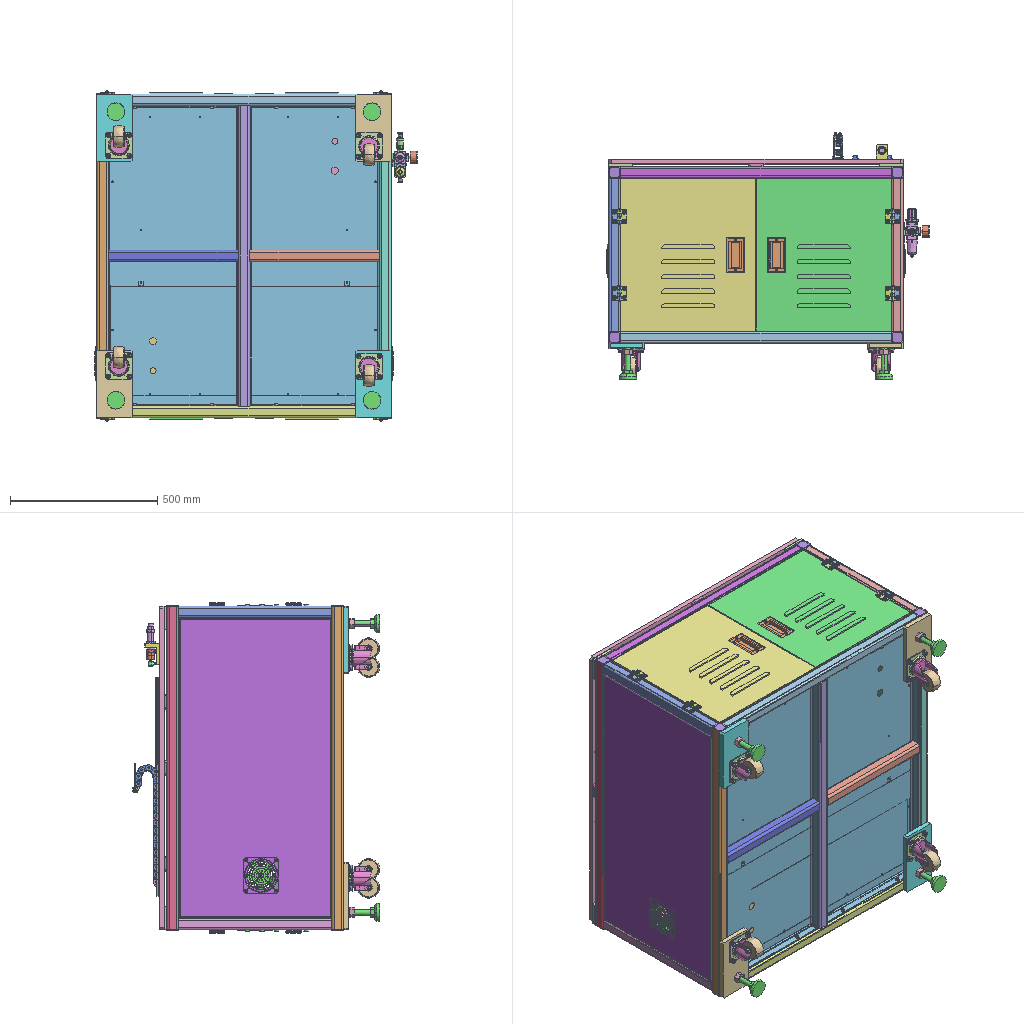Assembly | STEP file | 71 different items | 334 placed | box 1094 x 839 x 1122 mm
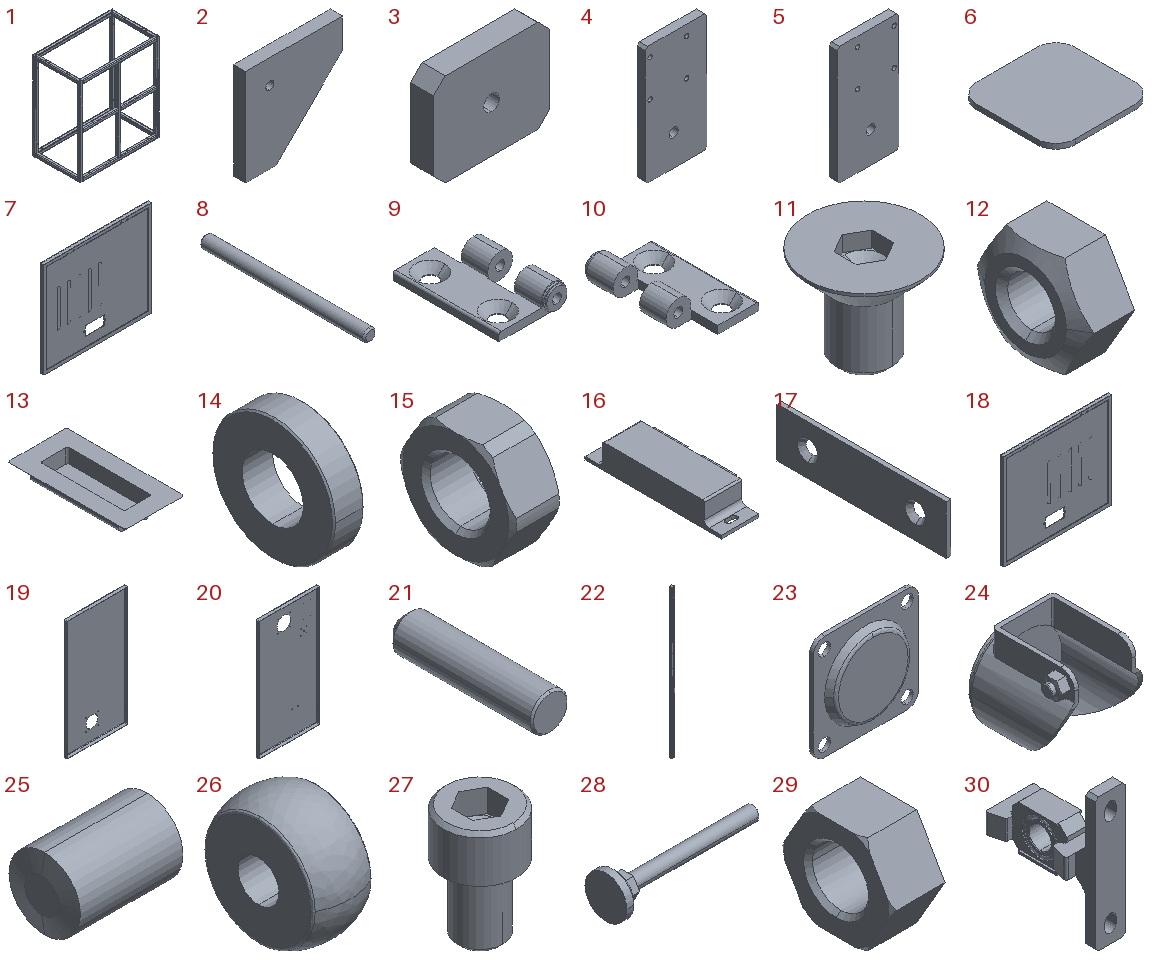Parts list (item | quantity | size | volume):
1 | x1 | 1000 x 600 x 1100 mm | 7334551 mm3
2 | x4 | 80 x 10 x 80 mm | 48512 mm3
3 | x5 | 50 x 10 x 40 mm | 19137 mm3
4 | x4 | 120 x 16 x 230 mm | 433239 mm3
5 | x4 | 120 x 16 x 230 mm | 433239 mm3
6 | x8 | 40 x 40 x 2 mm | 3090 mm3
7 | x2 | 520 x 20 x 460 mm | 497373 mm3
8 | x8 | 4 x 53.4 x 4 mm | 668.164 mm3
9 | x8 | 29.5 x 48.7 x 11 mm | 4677 mm3
10 | x8 | 29.5 x 48.7 x 11 mm | 4677 mm3
11 | x32 | 12 x 12 x 10 mm | 390.282 mm3
12 | x16 | 5 x 11.547 x 10 mm | 323.771 mm3
13 | x4 | 60 x 120 x 15 mm | 28231 mm3
14 | x8 | 2 x 8 x 8 mm | 75.149 mm3
15 | x8 | 3.2 x 7.66 x 7 mm | 92.29 mm3
16 | x8 | 26.5 x 86.5 x 15.5 mm | 25030 mm3
17 | x8 | 1.6 x 55 x 16 mm | 1334 mm3
18 | x2 | 520 x 20 x 460 mm | 497373 mm3
19 | x1 | 520 x 30 x 1020 mm | 905709 mm3
20 | x1 | 520 x 30 x 1020 mm | 901440 mm3
21 | x6 | 4 x 16 x 4 mm | 195.583 mm3
22 | x2 | 15 x 12.5 x 710 mm | 113515 mm3
23 | x4 | 90 x 9.6 x 90 mm | 43068 mm3
24 | x4 | 63.667 x 68.9 x 71.667 mm | 52181 mm3
25 | x4 | 38 x 25 x 25 mm | 18231 mm3
26 | x4 | 36 x 75 x 74.827 mm | 129062 mm3
27 | x16 | 16 x 16 x 25 mm | 2845 mm3
28 | x4 | 211 x 60 x 60 mm | 110948 mm3
29 | x4 | 16 x 34.641 x 30 mm | 8601 mm3
30 | x1 | 23.994 x 51.149 x 66 mm | 13543 mm3
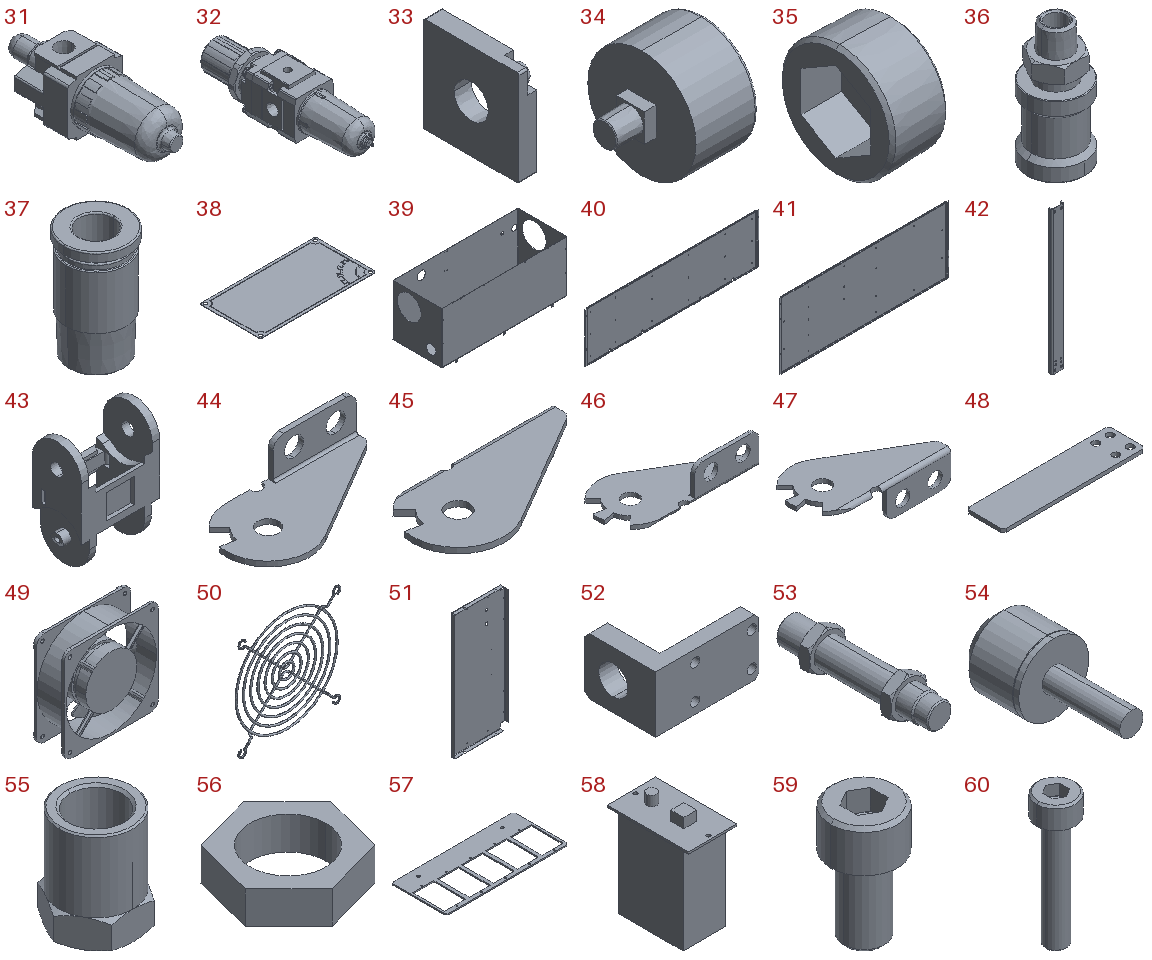31 | x1 | 40 x 119 x 40 mm | 93159 mm3
32 | x1 | 42.5 x 165.1 x 47 mm | 170625 mm3
33 | x2 | 5 x 27.1 x 27.1 mm | 3152 mm3
34 | x1 | 38.5 x 42 x 42 mm | 33324 mm3
35 | x1 | 5 x 9.772 x 9.772 mm | 252.752 mm3
36 | x1 | 26 x 26 x 58 mm | 16455 mm3
37 | x2 | 15 x 15 x 25.7 mm | 2155 mm3
38 | x1 | 126.7 x 66.1 x 0.4 mm | 3280 mm3
39 | x1 | 915 x 360 x 390 mm | 2426206 mm3
40 | x1 | 904 x 7 x 258 mm | 482267 mm3
41 | x1 | 900 x 8 x 353 mm | 657092 mm3
42 | x1 | 38 x 11.5 x 445 mm | 36734 mm3
43 | x19 | 32 x 20 x 45 mm | 6516 mm3
44 | x1 | 40 x 20 x 10 mm | 758.925 mm3
45 | x1 | 40 x 20 x 10 mm | 758.925 mm3
46 | x1 | 40 x 20 x 10 mm | 737.758 mm3
47 | x1 | 40 x 20 x 10 mm | 737.759 mm3
48 | x1 | 100 x 26 x 2.5 mm | 6284 mm3
49 | x2 | 120 x 38.9 x 120 mm | 179083 mm3
50 | x2 | 113.8 x 6.3 x 113.8 mm | 4425 mm3
51 | x2 | 440 x 30 x 1018 mm | 774968 mm3
52 | x1 | 73 x 50 x 40 mm | 44175 mm3
53 | x1 | 26 x 110 x 30.022 mm | 37581 mm3
54 | x1 | 18 x 35.8 x 18 mm | 4359 mm3
55 | x1 | 30.022 x 26 x 35 mm | 9758 mm3
56 | x2 | 28.896 x 29.097 x 8 mm | 2533 mm3
57 | x1 | 315 x 141 x 3 mm | 66219 mm3
58 | x5 | 60 x 100 x 124.5 mm | 482230 mm3
59 | x9 | 13 x 13 x 23 mm | 1660 mm3
60 | x24 | 5.5 x 5.5 x 19 mm | 174.028 mm3
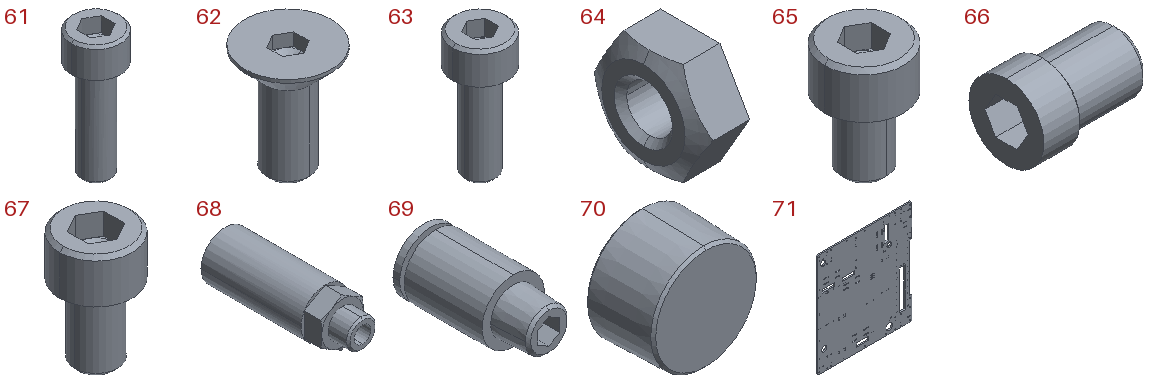61 | x4 | 10 x 10 x 26 mm | 955.225 mm3
62 | x4 | 8 x 8 x 10 mm | 162.002 mm3
63 | x4 | 7 x 7 x 16 mm | 284.727 mm3
64 | x4 | 3.2 x 8.083 x 7 mm | 104.501 mm3
65 | x19 | 7 x 7 x 10 mm | 209.329 mm3
66 | x12 | 15 x 10 x 10 mm | 791.764 mm3
67 | x2 | 10 x 10 x 16 mm | 672.482 mm3
68 | x2 | 22 x 63 x 22 mm | 20442 mm3
69 | x1 | 14 x 28 x 14 mm | 2474 mm3
70 | x3 | 13.263 x 8 x 13.263 mm | 903.778 mm3
71 | x1 | 1000 x 15 x 1100 mm | 15184573 mm3
Placements (level | parent | child | x y z in mm | rotation matrix by rows):
1 | subassembly 2 | subassembly 3 | -0.0 -0.0 -0.0 | 1 0 0 0 1 0 0 0 1
1 | subassembly 2 | subassembly 4 | -460.0 30.0 510.0 | 0 0 -1 0 -1 0 -1 0 0
1 | subassembly 2 | subassembly 4 | -460.0 30.0 -510.0 | 1 0 0 0 -1 0 0 0 -1
1 | subassembly 2 | subassembly 4 | 460.0 30.0 510.0 | -1 0 0 0 -1 0 0 0 1
1 | subassembly 2 | subassembly 4 | 460.0 30.0 -510.0 | 0 0 1 0 -1 0 1 0 0
1 | subassembly 2 | subassembly 5 | -0.0 30.0 -530.0 | 1 0 0 0 -1 0 0 0 -1
1 | subassembly 2 | subassembly 5 | -0.0 30.0 530.0 | -1 0 0 0 -1 0 0 0 1
1 | subassembly 2 | subassembly 5 | 480.0 20.0 -325.0 | 0 0 1 0 1 0 -1 0 0
1 | subassembly 2 | subassembly 5 | 480.0 20.0 225.0 | 0 0 -1 0 1 0 1 0 0
1 | subassembly 2 | subassembly 5 | -480.0 30.0 0.0 | 0 0 -1 0 -1 0 -1 0 0
1 | subassembly 2 | subassembly 6 | -440.0 -596.0 435.0 | -1 0 0 0 1 0 0 0 -1
1 | subassembly 2 | subassembly 6 | 440.0 -596.0 -435.0 | 1 0 0 0 1 0 0 0 1
1 | subassembly 2 | subassembly 7 | -440.0 -596.0 -435.0 | 1 0 0 0 1 0 0 0 1
1 | subassembly 2 | subassembly 7 | 440.0 -596.0 435.0 | -1 0 0 0 1 0 0 0 -1
1 | subassembly 2 | subassembly 8 | 480.0 -0.0 550.0 | 1 0 0 0 1 0 0 0 1
1 | subassembly 2 | subassembly 8 | 480.0 -560.0 550.0 | 1 0 0 0 1 0 0 0 1
1 | subassembly 2 | subassembly 8 | -480.0 -560.0 550.0 | 1 0 0 0 1 0 0 0 1
1 | subassembly 2 | subassembly 8 | -480.0 -0.0 550.0 | 1 0 0 0 1 0 0 0 1
1 | subassembly 2 | subassembly 8 | 480.0 -560.0 -552.0 | -1 0 0 0 -1 0 0 0 1
1 | subassembly 2 | subassembly 8 | 480.0 -0.0 -550.0 | -1 0 0 0 1 0 0 0 -1
1 | subassembly 2 | subassembly 8 | -480.0 -0.0 -552.0 | 0 1 0 -1 0 0 0 0 1
1 | subassembly 2 | subassembly 8 | -480.0 -560.0 -550.0 | -1 0 0 0 1 0 0 0 -1
1 | subassembly 2 | subassembly 9 | 230.0 -280.0 535.0 | 0 0 1 1 0 0 0 1 0
1 | subassembly 2 | subassembly 10 | 464.0 -410.0 555.5 | -0.9918 0 0.128 0 -1 0 0.128 0 0.9918
1 | subassembly 2 | subassembly 11 | 464.0 -410.0 555.5 | -1 0 0 0 -1 0 0 0 1
1 | subassembly 2 | subassembly 12 | 464.0 -410.0 555.5 | -1 0 0 0 -1 0 0 0 1
1 | subassembly 2 | subassembly 13 | 480.0 -425.0 550.2 | -1 0 0 0 -1 0 0 0 1
1 | subassembly 2 | subassembly 13 | 480.0 -395.0 550.2 | -1 0 0 0 -1 0 0 0 1
1 | subassembly 2 | subassembly 13 | 448.0 -395.0 550.2 | -1 0 0 0 -1 0 0 0 1
1 | subassembly 2 | subassembly 13 | 448.0 -425.0 550.2 | -1 0 0 0 -1 0 0 0 1
1 | subassembly 2 | subassembly 14 | 448.0 -425.0 548.8 | 0 0.9997 0.02547 0 -0.02547 0.9997 1 0 0
1 | subassembly 2 | subassembly 14 | 448.0 -395.0 548.8 | 0 0 1 0 -1 0 1 0 0
1 | subassembly 2 | subassembly 10 | 464.0 -150.0 555.5 | -0.9918 0 0.128 0 -1 0 0.128 0 0.9918
1 | subassembly 2 | subassembly 11 | 464.0 -150.0 555.5 | -1 0 0 0 -1 0 0 0 1
1 | subassembly 2 | subassembly 12 | 464.0 -150.0 555.5 | -1 0 0 0 -1 0 0 0 1
1 | subassembly 2 | subassembly 13 | 480.0 -165.0 550.2 | -1 0 0 0 -1 0 0 0 1
1 | subassembly 2 | subassembly 13 | 480.0 -135.0 550.2 | -1 0 0 0 -1 0 0 0 1
1 | subassembly 2 | subassembly 13 | 448.0 -135.0 550.2 | -1 0 0 0 -1 0 0 0 1
1 | subassembly 2 | subassembly 13 | 448.0 -165.0 550.2 | -1 0 0 0 -1 0 0 0 1
1 | subassembly 2 | subassembly 14 | 448.0 -165.0 548.8 | 0 0.9997 0.02547 0 -0.02547 0.9997 1 0 0
1 | subassembly 2 | subassembly 14 | 448.0 -135.0 548.8 | 0 0 1 0 -1 0 1 0 0
1 | subassembly 2 | subassembly 15 | 70.0 -280.0 550.0 | -1 0 0 0 -1 0 0 0 1
1 | subassembly 2 | subassembly 16 | 70.0 -330.0 546.8 | 0 0.723 0.6908 0 0.6908 -0.723 -1 0 0
1 | subassembly 2 | subassembly 17 | 70.0 -330.0 550.0 | 0 -0.4018 0.9157 0 0.9157 0.4018 -1 0 0
1 | subassembly 2 | subassembly 16 | 70.0 -230.0 550.0 | 0 0 1 0 1 0 -1 0 0
1 | subassembly 2 | subassembly 17 | 70.0 -230.0 548.0 | 0 0 1 0 1 0 -1 0 0
1 | subassembly 2 | subassembly 18 | 48.25 -19.5 518.65 | 0 -1 0 0 0 -1 1 0 0
1 | subassembly 2 | subassembly 19 | 48.25 -27.5 533.4 | 0 -1 0 0 0 -1 1 0 0
1 | subassembly 2 | subassembly 18 | 48.25 -540.5 518.65 | 0 1 0 0 0 1 1 0 0
1 | subassembly 2 | subassembly 19 | 48.25 -532.5 533.4 | 0 1 0 0 0 1 1 0 0
1 | subassembly 2 | subassembly 20 | -230.0 -280.0 535.0 | 0 0 -1 -1 0 0 0 1 0
1 | subassembly 2 | subassembly 10 | -464.0 -150.0 555.5 | 0.9918 0 -0.128 0 1 0 0.128 0 0.9918
1 | subassembly 2 | subassembly 11 | -464.0 -150.0 555.5 | 1 0 0 0 1 0 0 0 1
1 | subassembly 2 | subassembly 12 | -464.0 -150.0 555.5 | 1 0 0 0 1 0 0 0 1
1 | subassembly 2 | subassembly 13 | -480.0 -135.0 550.2 | 1 0 0 0 1 0 0 0 1
1 | subassembly 2 | subassembly 13 | -480.0 -165.0 550.2 | 1 0 0 0 1 0 0 0 1
1 | subassembly 2 | subassembly 13 | -448.0 -165.0 550.2 | 1 0 0 0 1 0 0 0 1
1 | subassembly 2 | subassembly 13 | -448.0 -135.0 550.2 | 1 0 0 0 1 0 0 0 1
1 | subassembly 2 | subassembly 14 | -448.0 -135.0 548.8 | 0 -0.9997 -0.02547 0 0.02547 -0.9997 1 0 0
1 | subassembly 2 | subassembly 14 | -448.0 -165.0 548.8 | 0 0 -1 0 1 0 1 0 0
1 | subassembly 2 | subassembly 10 | -464.0 -410.0 555.5 | 0.9918 0 -0.128 0 1 0 0.128 0 0.9918
1 | subassembly 2 | subassembly 11 | -464.0 -410.0 555.5 | 1 0 0 0 1 0 0 0 1
1 | subassembly 2 | subassembly 12 | -464.0 -410.0 555.5 | 1 0 0 0 1 0 0 0 1
1 | subassembly 2 | subassembly 13 | -480.0 -395.0 550.2 | 1 0 0 0 1 0 0 0 1
1 | subassembly 2 | subassembly 13 | -480.0 -425.0 550.2 | 1 0 0 0 1 0 0 0 1
1 | subassembly 2 | subassembly 13 | -448.0 -425.0 550.2 | 1 0 0 0 1 0 0 0 1
1 | subassembly 2 | subassembly 13 | -448.0 -395.0 550.2 | 1 0 0 0 1 0 0 0 1
1 | subassembly 2 | subassembly 14 | -448.0 -395.0 548.8 | 0 -0.9997 -0.02547 0 0.02547 -0.9997 1 0 0
1 | subassembly 2 | subassembly 14 | -448.0 -425.0 548.8 | 0 0 -1 0 1 0 1 0 0
1 | subassembly 2 | subassembly 15 | -70.0 -280.0 550.0 | 1 0 0 0 1 0 0 0 1
1 | subassembly 2 | subassembly 16 | -70.0 -230.0 546.8 | 0 -0.723 -0.6908 0 -0.6908 0.723 -1 0 0
1 | subassembly 2 | subassembly 17 | -70.0 -230.0 550.0 | 0 0.4018 -0.9157 0 -0.9157 -0.4018 -1 0 0
1 | subassembly 2 | subassembly 16 | -70.0 -330.0 550.0 | 0 0 -1 0 -1 0 -1 0 0
1 | subassembly 2 | subassembly 17 | -70.0 -330.0 548.0 | 0 0 -1 0 -1 0 -1 0 0
1 | subassembly 2 | subassembly 18 | -48.25 -540.5 518.65 | 0 1 0 0 0 1 1 0 0
1 | subassembly 2 | subassembly 19 | -48.25 -532.5 533.4 | 0 1 0 0 0 1 1 0 0
1 | subassembly 2 | subassembly 18 | -48.25 -19.5 518.65 | 0 -1 0 0 0 -1 1 0 0
1 | subassembly 2 | subassembly 19 | -48.25 -27.5 533.4 | 0 -1 0 0 0 -1 1 0 0
1 | subassembly 2 | subassembly 9 | -230.0 -280.0 -535.0 | 0 0 -1 1 0 0 0 -1 0
1 | subassembly 2 | subassembly 10 | -464.0 -410.0 -555.5 | 0.9918 0 -0.128 0 -1 0 -0.128 0 -0.9918
1 | subassembly 2 | subassembly 11 | -464.0 -410.0 -555.5 | 1 0 0 0 -1 0 0 0 -1
1 | subassembly 2 | subassembly 12 | -464.0 -410.0 -555.5 | 1 0 0 0 -1 0 0 0 -1
1 | subassembly 2 | subassembly 13 | -480.0 -425.0 -550.2 | 1 0 0 0 -1 0 0 0 -1
1 | subassembly 2 | subassembly 13 | -480.0 -395.0 -550.2 | 1 0 0 0 -1 0 0 0 -1
1 | subassembly 2 | subassembly 13 | -448.0 -395.0 -550.2 | 1 0 0 0 -1 0 0 0 -1
1 | subassembly 2 | subassembly 13 | -448.0 -425.0 -550.2 | 1 0 0 0 -1 0 0 0 -1
1 | subassembly 2 | subassembly 14 | -448.0 -425.0 -548.8 | 0 -0.9997 -0.02547 0 -0.02547 0.9997 -1 0 0
1 | subassembly 2 | subassembly 14 | -448.0 -395.0 -548.8 | 0 0 -1 0 -1 0 -1 0 0
1 | subassembly 2 | subassembly 10 | -464.0 -150.0 -555.5 | 0.9918 0 -0.128 0 -1 0 -0.128 0 -0.9918
1 | subassembly 2 | subassembly 11 | -464.0 -150.0 -555.5 | 1 0 0 0 -1 0 0 0 -1
1 | subassembly 2 | subassembly 12 | -464.0 -150.0 -555.5 | 1 0 0 0 -1 0 0 0 -1
1 | subassembly 2 | subassembly 13 | -480.0 -165.0 -550.2 | 1 0 0 0 -1 0 0 0 -1
1 | subassembly 2 | subassembly 13 | -480.0 -135.0 -550.2 | 1 0 0 0 -1 0 0 0 -1
1 | subassembly 2 | subassembly 13 | -448.0 -135.0 -550.2 | 1 0 0 0 -1 0 0 0 -1
1 | subassembly 2 | subassembly 13 | -448.0 -165.0 -550.2 | 1 0 0 0 -1 0 0 0 -1
1 | subassembly 2 | subassembly 14 | -448.0 -165.0 -548.8 | 0 -0.9997 -0.02547 0 -0.02547 0.9997 -1 0 0
1 | subassembly 2 | subassembly 14 | -448.0 -135.0 -548.8 | 0 0 -1 0 -1 0 -1 0 0
1 | subassembly 2 | subassembly 15 | -70.0 -280.0 -550.0 | 1 0 0 0 -1 0 0 0 -1
1 | subassembly 2 | subassembly 16 | -70.0 -330.0 -546.8 | 0 -0.723 -0.6908 0 0.6908 -0.723 1 0 0
1 | subassembly 2 | subassembly 17 | -70.0 -330.0 -550.0 | 0 0.4018 -0.9157 0 0.9157 0.4018 1 0 0
1 | subassembly 2 | subassembly 16 | -70.0 -230.0 -550.0 | 0 0 -1 0 1 0 1 0 0
1 | subassembly 2 | subassembly 17 | -70.0 -230.0 -548.0 | 0 0 -1 0 1 0 1 0 0
1 | subassembly 2 | subassembly 18 | -48.25 -19.5 -518.65 | 0 1 0 0 0 -1 -1 0 0
1 | subassembly 2 | subassembly 19 | -48.25 -27.5 -533.4 | 0 1 0 0 0 -1 -1 0 0
1 | subassembly 2 | subassembly 18 | -48.25 -540.5 -518.65 | 0 -1 0 0 0 1 -1 0 0
1 | subassembly 2 | subassembly 19 | -48.25 -532.5 -533.4 | 0 -1 0 0 0 1 -1 0 0
1 | subassembly 2 | subassembly 20 | 230.0 -280.0 -535.0 | 0 0 1 -1 0 0 0 -1 0
1 | subassembly 2 | subassembly 10 | 464.0 -150.0 -555.5 | -0.9918 0 0.128 0 1 0 -0.128 0 -0.9918
1 | subassembly 2 | subassembly 11 | 464.0 -150.0 -555.5 | -1 0 0 0 1 0 0 0 -1
1 | subassembly 2 | subassembly 12 | 464.0 -150.0 -555.5 | -1 0 0 0 1 0 0 0 -1
1 | subassembly 2 | subassembly 13 | 480.0 -135.0 -550.2 | -1 0 0 0 1 0 0 0 -1
1 | subassembly 2 | subassembly 13 | 480.0 -165.0 -550.2 | -1 0 0 0 1 0 0 0 -1
1 | subassembly 2 | subassembly 13 | 448.0 -165.0 -550.2 | -1 0 0 0 1 0 0 0 -1
1 | subassembly 2 | subassembly 13 | 448.0 -135.0 -550.2 | -1 0 0 0 1 0 0 0 -1
1 | subassembly 2 | subassembly 14 | 448.0 -135.0 -548.8 | 0 0.9997 0.02547 0 0.02547 -0.9997 -1 0 0
1 | subassembly 2 | subassembly 14 | 448.0 -165.0 -548.8 | 0 0 1 0 1 0 -1 0 0
1 | subassembly 2 | subassembly 10 | 464.0 -410.0 -555.5 | -0.9918 0 0.128 0 1 0 -0.128 0 -0.9918
1 | subassembly 2 | subassembly 11 | 464.0 -410.0 -555.5 | -1 0 0 0 1 0 0 0 -1
1 | subassembly 2 | subassembly 12 | 464.0 -410.0 -555.5 | -1 0 0 0 1 0 0 0 -1
1 | subassembly 2 | subassembly 13 | 480.0 -395.0 -550.2 | -1 0 0 0 1 0 0 0 -1
1 | subassembly 2 | subassembly 13 | 480.0 -425.0 -550.2 | -1 0 0 0 1 0 0 0 -1
1 | subassembly 2 | subassembly 13 | 448.0 -425.0 -550.2 | -1 0 0 0 1 0 0 0 -1
1 | subassembly 2 | subassembly 13 | 448.0 -395.0 -550.2 | -1 0 0 0 1 0 0 0 -1
1 | subassembly 2 | subassembly 14 | 448.0 -395.0 -548.8 | 0 0.9997 0.02547 0 0.02547 -0.9997 -1 0 0
1 | subassembly 2 | subassembly 14 | 448.0 -425.0 -548.8 | 0 0 1 0 1 0 -1 0 0
1 | subassembly 2 | subassembly 15 | 70.0 -280.0 -550.0 | -1 0 0 0 1 0 0 0 -1
1 | subassembly 2 | subassembly 16 | 70.0 -230.0 -546.8 | 0 0.723 0.6908 0 -0.6908 0.723 1 0 0
1 | subassembly 2 | subassembly 17 | 70.0 -230.0 -550.0 | 0 -0.4018 0.9157 0 -0.9157 -0.4018 1 0 0
1 | subassembly 2 | subassembly 16 | 70.0 -330.0 -550.0 | 0 0 1 0 -1 0 1 0 0
1 | subassembly 2 | subassembly 17 | 70.0 -330.0 -548.0 | 0 0 1 0 -1 0 1 0 0
1 | subassembly 2 | subassembly 18 | 48.25 -540.5 -518.65 | 0 -1 0 0 0 1 -1 0 0
1 | subassembly 2 | subassembly 19 | 48.25 -532.5 -533.4 | 0 -1 0 0 0 1 -1 0 0
1 | subassembly 2 | subassembly 18 | 48.25 -19.5 -518.65 | 0 1 0 0 0 -1 -1 0 0
1 | subassembly 2 | subassembly 19 | 48.25 -27.5 -533.4 | 0 1 0 0 0 -1 -1 0 0
1 | subassembly 2 | subassembly 21 | -470.0 -280.0 -0.0 | 0 -1 0 1 0 0 0 0 1
1 | subassembly 2 | subassembly 22 | 470.0 -280.0 -0.0 | 0 1 0 1 0 0 0 0 -1
1 | subassembly 2 | subassembly 23 | 462.0 33.0 -385.0 | 0.9252 0 0.3796 0 1 0 -0.3796 0 0.9252
1 | subassembly 2 | subassembly 23 | 346.0 33.0 -385.0 | 0.9252 0 0.3796 0 1 0 -0.3796 0 0.9252
1 | subassembly 2 | subassembly 23 | 346.0 33.0 -75.0 | 1 0 0 0 1 0 0 0 1
1 | subassembly 2 | subassembly 23 | 346.0 33.0 235.0 | 1 0 0 0 1 0 0 0 1
1 | subassembly 2 | subassembly 23 | 462.0 33.0 -75.0 | 1 0 0 0 1 0 0 0 1
1 | subassembly 2 | subassembly 23 | 462.0 33.0 235.0 | 1 0 0 0 1 0 0 0 1
1 | subassembly 2 | subassembly 24 | 452.5 69.0 -363.0 | 1 0 0 0 1 0 0 0 1
1 | subassembly 2 | subassembly 24 | 336.5 69.0 -363.0 | 1 0 0 0 1 0 0 0 1
1 | subassembly 2 | subassembly 6 | 440.0 -596.0 -435.0 | 1 0 0 0 1 0 0 0 1
1 | subassembly 2 | subassembly 25 | 425.0 -596.0 -375.866 | -1 0 0 0 1 0 0 0 -1
1 | subassembly 2 | subassembly 26 | 425.0 -596.0 -375.866 | -1 0 0 0 1 0 0 0 -1
1 | subassembly 2 | subassembly 27 | 425.0 -664.5 -405.866 | 1 0 0 0 -1 0 0 0 -1
1 | subassembly 2 | subassembly 28 | 425.0 -664.5 -405.866 | -1 0 0 0 1 0 0 0 -1
1 | subassembly 2 | subassembly 29 | 389.5 -599.2 -411.366 | -1 0 0 0 0 -1 0 -1 0
1 | subassembly 2 | subassembly 29 | 389.5 -599.2 -340.366 | -1 0 0 0 0 -1 0 -1 0
1 | subassembly 2 | subassembly 29 | 460.5 -599.2 -340.366 | -1 0 0 0 0 -1 0 -1 0
1 | subassembly 2 | subassembly 29 | 460.5 -599.2 -411.366 | -1 0 0 0 0 -1 0 -1 0
1 | subassembly 2 | subassembly 30 | 435.0 -702.0 -490.0 | 0 0.9914 0.1311 1 0 0 0 0.1311 -0.9914
1 | subassembly 2 | subassembly 31 | 435.0 -617.0 -490.0 | 0 0.987 0.1607 1 0 0 0 0.1607 -0.987
1 | subassembly 2 | subassembly 7 | 440.0 -596.0 435.0 | -1 0 0 0 1 0 0 0 -1
1 | subassembly 2 | subassembly 25 | 425.0 -596.0 373.5 | -1 0 0 0 1 0 0 0 -1
1 | subassembly 2 | subassembly 26 | 425.0 -596.0 373.5 | -1 0 0 0 1 0 0 0 -1
1 | subassembly 2 | subassembly 27 | 425.0 -664.5 343.5 | 1 0 0 0 -1 0 0 0 -1
1 | subassembly 2 | subassembly 28 | 425.0 -664.5 343.5 | -1 0 0 0 1 0 0 0 -1
1 | subassembly 2 | subassembly 29 | 389.5 -599.2 338.0 | -1 0 0 0 0 -1 0 -1 0
1 | subassembly 2 | subassembly 29 | 389.5 -599.2 409.0 | -1 0 0 0 0 -1 0 -1 0
1 | subassembly 2 | subassembly 29 | 460.5 -599.2 409.0 | -1 0 0 0 0 -1 0 -1 0
1 | subassembly 2 | subassembly 29 | 460.5 -599.2 338.0 | -1 0 0 0 0 -1 0 -1 0
1 | subassembly 2 | subassembly 30 | 435.0 -702.0 490.0 | 0 0 1 1 0 0 0 1 0
1 | subassembly 2 | subassembly 31 | 435.0 -617.0 490.0 | 0 -0.02991 0.9996 1 0 0 0 0.9996 0.02991
1 | subassembly 2 | subassembly 6 | -440.0 -596.0 435.0 | -1 0 0 0 1 0 0 0 -1
1 | subassembly 2 | subassembly 25 | -425.0 -596.0 375.866 | 1 0 0 0 1 0 0 0 1
1 | subassembly 2 | subassembly 26 | -425.0 -596.0 375.866 | 1 0 0 0 1 0 0 0 1
1 | subassembly 2 | subassembly 27 | -425.0 -664.5 405.866 | -1 0 0 0 -1 0 0 0 1
1 | subassembly 2 | subassembly 28 | -425.0 -664.5 405.866 | 1 0 0 0 1 0 0 0 1
1 | subassembly 2 | subassembly 29 | -389.5 -599.2 411.366 | 1 0 0 0 0 -1 0 1 0
1 | subassembly 2 | subassembly 29 | -389.5 -599.2 340.366 | 1 0 0 0 0 -1 0 1 0
1 | subassembly 2 | subassembly 29 | -460.5 -599.2 340.366 | 1 0 0 0 0 -1 0 1 0
1 | subassembly 2 | subassembly 29 | -460.5 -599.2 411.366 | 1 0 0 0 0 -1 0 1 0
1 | subassembly 2 | subassembly 30 | -435.0 -702.0 490.0 | 0 -0.9914 -0.1311 1 0 0 0 -0.1311 0.9914
1 | subassembly 2 | subassembly 31 | -435.0 -617.0 490.0 | 0 -0.987 -0.1607 1 0 0 0 -0.1607 0.987
1 | subassembly 2 | subassembly 7 | -440.0 -596.0 -435.0 | 1 0 0 0 1 0 0 0 1
1 | subassembly 2 | subassembly 25 | -425.0 -596.0 -373.5 | 1 0 0 0 1 0 0 0 1
1 | subassembly 2 | subassembly 26 | -425.0 -596.0 -373.5 | 1 0 0 0 1 0 0 0 1
1 | subassembly 2 | subassembly 27 | -425.0 -664.5 -343.5 | -1 0 0 0 -1 0 0 0 1
1 | subassembly 2 | subassembly 28 | -425.0 -664.5 -343.5 | 1 0 0 0 1 0 0 0 1
1 | subassembly 2 | subassembly 29 | -389.5 -599.2 -338.0 | 1 0 0 0 0 -1 0 1 0
1 | subassembly 2 | subassembly 29 | -389.5 -599.2 -409.0 | 1 0 0 0 0 -1 0 1 0
1 | subassembly 2 | subassembly 29 | -460.5 -599.2 -409.0 | 1 0 0 0 0 -1 0 1 0
1 | subassembly 2 | subassembly 29 | -460.5 -599.2 -338.0 | 1 0 0 0 0 -1 0 1 0
1 | subassembly 2 | subassembly 30 | -435.0 -702.0 -490.0 | 0 0 -1 1 0 0 0 -1 0
1 | subassembly 2 | subassembly 31 | -435.0 -617.0 -490.0 | 0 0.02991 -0.9996 1 0 0 0 -0.9996 -0.02991
1 | subassembly 2 | subassembly 32 | 500.0 -203.5 310.0 | 0 1 0 0 0 -1 -1 0 0
1 | subassembly 2 | subassembly 33 | 530.0 -226.5 285.0 | 1 0 0 0 1 0 0 0 1
1 | subassembly 2 | subassembly 34 | 530.0 -171.0 335.0 | 0 0 1 0 1 0 -1 0 0
1 | subassembly 2 | subassembly 35 | 558.5 -199.5 335.0 | 1 0 0 0 1 0 0 0 1
1 | subassembly 2 | subassembly 36 | 588.0 -199.5 335.0 | 1 0 0 0 1 0 0 0 1
1 | subassembly 2 | subassembly 35 | 501.5 -199.5 335.0 | -1 0 0 0 -1 0 0 0 1
1 | subassembly 2 | subassembly 37 | 502.0 -199.5 335.0 | 1 0 0 0 1 0 0 0 1
1 | subassembly 2 | subassembly 38 | 530.0 -203.5 343.5 | -0.9347 -0.3555 0 -0.3555 0.9347 0 0 0 -1
1 | subassembly 2 | subassembly 39 | 530.0 -203.5 392.5 | 1 0 0 0 1 0 0 0 1
1 | subassembly 2 | subassembly 39 | 530.0 -203.5 274.0 | -0.9237 -0.383 0 -0.383 0.9237 0 0 0 -1
1 | subassembly 2 | subassembly 40 | 500.4 -103.05 -366.65 | 0 0 1 0 1 0 -1 0 0
1 | subassembly 2 | subassembly 41 | -0.0 -360.0 -100.0 | -1 0 0 0 1 0 0 0 -1
1 | subassembly 2 | subassembly 42 | -0.0 -531.0 -348.0 | 1 0 0 0 1 0 0 0 1
1 | subassembly 2 | subassembly 43 | -0.0 -360.0 -110.0 | 1 0 0 0 0 1 0 -1 0
1 | subassembly 2 | subassembly 44 | 278.0 46.5 -212.5 | 1 0 0 0 1 0 0 0 1
1 | subassembly 2 | subassembly 45 | 278.0 116.5 -63.443 | 1 0 0 0 -1 0 0 0 -1
1 | subassembly 2 | subassembly 45 | 278.0 120.667 -37.533 | 1 0 0 0 -0.9091 0.4167 0 -0.4167 -0.9091
1 | subassembly 2 | subassembly 45 | 278.0 115.69 -8.494 | 1 0 0 0 -0.2778 0.9606 0 -0.9606 -0.2778
1 | subassembly 2 | subassembly 45 | 278.0 90.442 6.692 | 1 0 0 0 0.5464 0.8375 0 -0.8375 0.5464
1 | subassembly 2 | subassembly 45 | 278.0 62.981 -2.605 | 1 0 0 0 0.9827 0.1852 0 -0.1852 0.9827
1 | subassembly 2 | subassembly 45 | 278.0 56.5 -27.0 | 1 0 0 0 1 0 0 0 1
1 | subassembly 2 | subassembly 45 | 278.0 56.5 -52.0 | 1 0 0 0 1 0 0 0 1
1 | subassembly 2 | subassembly 45 | 278.0 56.5 -77.0 | 1 0 0 0 1 0 0 0 1
1 | subassembly 2 | subassembly 45 | 278.0 56.5 -102.0 | 1 0 0 0 1 0 0 0 1
1 | subassembly 2 | subassembly 45 | 278.0 56.5 -127.0 | 1 0 0 0 1 0 0 0 1
1 | subassembly 2 | subassembly 45 | 278.0 56.5 -152.0 | 1 0 0 0 1 0 0 0 1
1 | subassembly 2 | subassembly 45 | 278.0 56.5 -177.0 | 1 0 0 0 1 0 0 0 1
1 | subassembly 2 | subassembly 45 | 278.0 56.5 -202.0 | 1 0 0 0 1 0 0 0 1
1 | subassembly 2 | subassembly 45 | 278.0 56.5 -227.0 | 1 0 0 0 1 0 0 0 1
1 | subassembly 2 | subassembly 45 | 278.0 56.5 -252.0 | 1 0 0 0 1 0 0 0 1
1 | subassembly 2 | subassembly 45 | 278.0 56.5 -277.0 | 1 0 0 0 1 0 0 0 1
1 | subassembly 2 | subassembly 45 | 278.0 56.5 -302.0 | 1 0 0 0 1 0 0 0 1
1 | subassembly 2 | subassembly 45 | 278.0 56.5 -327.0 | 1 0 0 0 1 0 0 0 1
1 | subassembly 2 | subassembly 45 | 278.0 56.5 -352.0 | 1 0 0 0 1 0 0 0 1
1 | subassembly 2 | subassembly 46 | 291.9 66.5 -387.0 | 0 0 -1 0 -1 0 -1 0 0
1 | subassembly 2 | subassembly 47 | 264.1 66.5 -387.0 | 0 0 -1 0 -1 0 -1 0 0
1 | subassembly 2 | subassembly 48 | 291.0 126.5 -53.443 | 0 0 -1 0 -1 0 -1 0 0
1 | subassembly 2 | subassembly 49 | 265.0 126.5 -53.443 | 0 0 -1 0 -1 0 -1 0 0
1 | subassembly 2 | subassembly 50 | 278.0 126.5 -33.443 | 0 -1 0 0 0 1 -1 0 0
1 | subassembly 2 | subassembly 51 | 487.6 -300.0 -365.0 | 0 1 0 0 0 -1 -1 0 0
1 | subassembly 2 | subassembly 52 | 489.6 -300.0 -365.0 | 0 1 0 0 0 -1 -1 0 0
1 | subassembly 2 | subassembly 51 | -487.6 -300.0 -365.0 | 0 -1 0 1 0 0 0 0 1
1 | subassembly 2 | subassembly 52 | -489.6 -300.0 -365.0 | 0 -1 0 1 0 0 0 0 1
1 | subassembly 2 | subassembly 53 | 240.0 -570.0 1.0 | 1 0 0 0 1 0 0 0 1
1 | subassembly 2 | subassembly 53 | -240.0 -570.0 -0.0 | -1 0 0 0 1 0 0 0 -1
1 | subassembly 2 | subassembly 54 | 428.0 55.0 410.0 | 0 0 1 0 1 0 -1 0 0
1 | subassembly 2 | subassembly 55 | 428.0 75.0 492.0 | 0.1382 0 0.9904 -0.9904 0 0.1382 0 -1 0
1 | subassembly 2 | subassembly 56 | 428.0 75.0 492.0 | 0.1382 0 0.9904 -0.9904 0 0.1382 0 -1 0
1 | subassembly 2 | subassembly 57 | 428.0 75.0 384.5 | 0.1382 -0.9904 0 -0.9904 -0.1382 0 0 0 -1
1 | subassembly 2 | subassembly 58 | 428.0 75.0 418.0 | -0.07756 -0.997 0 -0.997 0.07756 0 0 0 -1
1 | subassembly 2 | subassembly 58 | 428.0 75.0 431.0 | -1 0 0 0 1 0 0 0 -1
1 | subassembly 2 | subassembly 59 | -293.5 -40.0 -507.0 | -1 0 0 0 1 0 0 0 -1
1 | subassembly 2 | subassembly 60 | -169.0 -71.0 -510.0 | -1 0 0 0 1 0 0 0 -1
1 | subassembly 2 | subassembly 60 | -231.0 -71.0 -510.0 | -1 0 0 0 1 0 0 0 -1
1 | subassembly 2 | subassembly 60 | -293.0 -71.0 -510.0 | -1 0 0 0 1 0 0 0 -1
1 | subassembly 2 | subassembly 60 | -355.0 -71.0 -510.0 | -1 0 0 0 1 0 0 0 -1
1 | subassembly 2 | subassembly 60 | -417.0 -71.0 -510.0 | -1 0 0 0 1 0 0 0 -1
1 | subassembly 2 | subassembly 61 | 480.0 36.4 530.0 | 1 0 0 0 0 1 0 -1 0
1 | subassembly 2 | subassembly 61 | -480.0 36.4 -530.0 | 1 0 0 0 0 1 0 -1 0
1 | subassembly 2 | subassembly 61 | -0.0 36.4 -530.0 | 1 0 0 0 0 1 0 -1 0
1 | subassembly 2 | subassembly 61 | 480.0 36.4 -325.0 | 1 0 0 0 0 1 0 -1 0
1 | subassembly 2 | subassembly 61 | -0.0 36.4 530.0 | 1 0 0 0 0 1 0 -1 0
1 | subassembly 2 | subassembly 61 | -480.0 36.4 -0.0 | 1 0 0 0 0 1 0 -1 0
1 | subassembly 2 | subassembly 61 | -480.0 36.4 530.0 | 1 0 0 0 0 1 0 -1 0
1 | subassembly 2 | subassembly 61 | 480.0 36.4 225.0 | 1 0 0 0 0 1 0 -1 0
1 | subassembly 2 | subassembly 61 | 480.0 36.4 -530.0 | 1 0 0 0 0 1 0 -1 0
1 | subassembly 2 | subassembly 62 | 336.5 53.0 -388.0 | 0.326 -0.9454 0 0 0 1 -0.9454 -0.326 0
1 | subassembly 2 | subassembly 62 | 452.5 53.0 -388.0 | 0.326 -0.9454 0 0 0 1 -0.9454 -0.326 0
1 | subassembly 2 | subassembly 63 | 416.0 55.0 355.0 | 0.9391 -0.3436 0 0 0 1 -0.3436 -0.9391 0
1 | subassembly 2 | subassembly 63 | 440.0 55.0 355.0 | 0.9391 -0.3436 0 0 0 1 -0.3436 -0.9391 0
1 | subassembly 2 | subassembly 63 | 440.0 55.0 395.0 | 0.9391 -0.3436 0 0 0 1 -0.3436 -0.9391 0
1 | subassembly 2 | subassembly 63 | 416.0 55.0 395.0 | 0.9391 -0.3436 0 0 0 1 -0.3436 -0.9391 0
1 | subassembly 2 | subassembly 64 | 268.0 44.2 -425.0 | 0.7216 0.6923 0 0 0 1 0.6923 -0.7216 0
1 | subassembly 2 | subassembly 64 | 288.0 44.2 -425.0 | 0.7216 0.6923 0 0 0 1 0.6923 -0.7216 0
1 | subassembly 2 | subassembly 64 | 288.0 44.2 -0.0 | 0.7216 0.6923 0 0 0 1 0.6923 -0.7216 0
1 | subassembly 2 | subassembly 64 | 268.0 44.2 0.0 | 0.7216 0.6923 0 0 0 1 0.6923 -0.7216 0
1 | subassembly 2 | subassembly 65 | 285.0 125.3 -78.443 | -0.3569 -0.9341 0 0 0 -1 0.9341 -0.3569 0
1 | subassembly 2 | subassembly 65 | 271.0 125.3 -78.443 | -0.3569 -0.9341 0 0 0 -1 0.9341 -0.3569 0
1 | subassembly 2 | subassembly 65 | 285.0 125.3 -68.443 | -0.3569 -0.9341 0 0 0 -1 0.9341 -0.3569 0
1 | subassembly 2 | subassembly 65 | 271.0 125.3 -68.443 | -0.3569 -0.9341 0 0 0 -1 0.9341 -0.3569 0
1 | subassembly 2 | subassembly 66 | 285.0 132.0 -78.443 | 0 -0.3138 -0.9495 -1 0 0 0 0.9495 -0.3138
1 | subassembly 2 | subassembly 66 | 271.0 132.0 -68.443 | 0 -0.3138 -0.9495 -1 0 0 0 0.9495 -0.3138
1 | subassembly 2 | subassembly 66 | 285.0 132.0 -68.443 | 0 -0.3138 -0.9495 -1 0 0 0 0.9495 -0.3138
1 | subassembly 2 | subassembly 66 | 271.0 132.0 -78.443 | 0 0.8224 0.5689 -1 0 0 0 -0.5689 0.8224
1 | subassembly 2 | subassembly 67 | 270.1 47.7 -412.0 | 0.9918 0.128 0 0 0 1 0.128 -0.9918 0
1 | subassembly 2 | subassembly 67 | 285.9 47.7 -402.0 | 0.9918 0.128 0 0 0 1 0.128 -0.9918 0
1 | subassembly 2 | subassembly 67 | 285.9 47.7 -412.0 | 0.9918 0.128 0 0 0 1 0.128 -0.9918 0
1 | subassembly 2 | subassembly 67 | 270.1 47.7 -402.0 | 0.9918 0.128 0 0 0 1 0.128 -0.9918 0
1 | subassembly 2 | subassembly 68 | 480.0 -538.5 410.0 | 0 0.9216 -0.3883 -1 0 0 0 0.3883 0.9216
1 | subassembly 2 | subassembly 67 | -350.0 -538.0 -88.0 | 0.1339 -0.991 0 0 0 1 -0.991 -0.1339 0
1 | subassembly 2 | subassembly 67 | -320.0 -538.0 -470.0 | 0.1339 -0.991 0 0 0 1 -0.991 -0.1339 0
1 | subassembly 2 | subassembly 67 | 444.5 -280.0 -104.0 | 0.2459 -0.9693 0 -0.9693 -0.2459 0 0 0 -1
1 | subassembly 2 | subassembly 67 | 444.5 -440.0 -104.0 | -0.1325 -0.9912 0 -0.9912 0.1325 0 0 0 -1
1 | subassembly 2 | subassembly 67 | -444.5 -440.0 -104.0 | 0.05478 -0.9985 0 -0.9985 -0.05478 0 0 0 -1
1 | subassembly 2 | subassembly 67 | -444.5 -280.0 -104.0 | 0.5169 -0.8561 0 -0.8561 -0.5169 0 0 0 -1
1 | subassembly 2 | subassembly 67 | 447.0 -536.0 -401.0 | 1 0 0 0 0 1 0 -1 0
1 | subassembly 2 | subassembly 67 | 447.0 -536.0 -251.0 | 0.6313 -0.7756 0 0 0 1 -0.7756 -0.6313 0
1 | subassembly 2 | subassembly 67 | -447.0 -536.0 -251.0 | 0.6313 -0.7756 0 0 0 1 -0.7756 -0.6313 0
1 | subassembly 2 | subassembly 67 | -447.0 -536.0 -401.0 | 0.6313 -0.7756 0 0 0 1 -0.7756 -0.6313 0
1 | subassembly 2 | subassembly 67 | -150.0 -538.0 -470.0 | 0.6313 -0.7756 0 0 0 1 -0.7756 -0.6313 0
1 | subassembly 2 | subassembly 67 | 320.0 -538.0 -471.0 | 0.6313 -0.7756 0 0 0 1 -0.7756 -0.6313 0
1 | subassembly 2 | subassembly 67 | 150.0 -538.0 -471.0 | 0.6313 -0.7756 0 0 0 1 -0.7756 -0.6313 0
1 | subassembly 2 | subassembly 68 | -110.0 -562.0 507.5 | 0 0.8802 -0.4746 0 0.4746 0.8802 1 0 0
1 | subassembly 2 | subassembly 68 | 370.0 -562.0 507.5 | 0 0.9988 -0.04852 0 0.04852 0.9988 1 0 0
1 | subassembly 2 | subassembly 68 | 110.0 -562.0 507.5 | 0 0.7554 -0.6552 0 0.6552 0.7554 1 0 0
1 | subassembly 2 | subassembly 68 | -370.0 -562.0 507.5 | 0 0.9933 0.1158 0 -0.1158 0.9933 1 0 0
1 | subassembly 2 | subassembly 68 | 370.0 -562.0 -507.5 | 0 -0.9824 0.187 0 0.187 0.9824 -1 0 0
1 | subassembly 2 | subassembly 68 | 110.0 -562.0 -507.5 | 0 -0.5636 -0.826 0 -0.826 0.5636 -1 0 0
1 | subassembly 2 | subassembly 68 | -110.0 -562.0 -507.5 | 0 -0.6141 -0.7892 0 -0.7892 0.6141 -1 0 0
1 | subassembly 2 | subassembly 68 | -370.0 -562.0 -507.5 | 0 -0.2131 -0.977 0 -0.977 0.2131 -1 0 0
1 | subassembly 2 | subassembly 67 | 350.0 -538.0 -88.0 | 0.1339 -0.991 0 0 0 1 -0.991 -0.1339 0
1 | subassembly 2 | subassembly 67 | 0.0 -538.0 -88.0 | 0.1339 -0.991 0 0 0 1 -0.991 -0.1339 0
1 | subassembly 2 | subassembly 68 | 480.0 -538.5 -410.0 | 0 0.9216 -0.3883 -1 0 0 0 0.3883 0.9216
1 | subassembly 2 | subassembly 68 | -480.0 -538.5 410.0 | 0 0.9216 -0.3883 -1 0 0 0 0.3883 0.9216
1 | subassembly 2 | subassembly 68 | -480.0 -538.5 -410.0 | 0 0.9216 -0.3883 -1 0 0 0 0.3883 0.9216
1 | subassembly 2 | subassembly 69 | -401.0 -0.0 -507.0 | 1 0 0 0 1 0 0 0 1
1 | subassembly 2 | subassembly 69 | -186.0 -0.0 -507.0 | 1 0 0 0 1 0 0 0 1
1 | subassembly 2 | subassembly 62 | 452.5 53.0 -328.0 | 0.326 -0.9454 0 0 0 1 -0.9454 -0.326 0
1 | subassembly 2 | subassembly 62 | 452.5 53.0 -268.0 | 0.326 -0.9454 0 0 0 1 -0.9454 -0.326 0
1 | subassembly 2 | subassembly 62 | 452.5 53.0 -208.0 | 0.326 -0.9454 0 0 0 1 -0.9454 -0.326 0
1 | subassembly 2 | subassembly 62 | 452.5 53.0 -148.0 | 0.326 -0.9454 0 0 0 1 -0.9454 -0.326 0
1 | subassembly 2 | subassembly 62 | 452.5 53.0 -88.0 | 0.326 -0.9454 0 0 0 1 -0.9454 -0.326 0
1 | subassembly 2 | subassembly 62 | 452.5 53.0 -28.0 | 0.326 -0.9454 0 0 0 1 -0.9454 -0.326 0
1 | subassembly 2 | subassembly 62 | 452.5 53.0 32.0 | 0.326 -0.9454 0 0 0 1 -0.9454 -0.326 0
1 | subassembly 2 | subassembly 62 | 452.5 53.0 92.0 | 0.326 -0.9454 0 0 0 1 -0.9454 -0.326 0
1 | subassembly 2 | subassembly 62 | 452.5 53.0 152.0 | 0.326 -0.9454 0 0 0 1 -0.9454 -0.326 0
1 | subassembly 2 | subassembly 62 | 452.5 53.0 212.0 | 0.326 -0.9454 0 0 0 1 -0.9454 -0.326 0
1 | subassembly 2 | subassembly 62 | 452.5 53.0 272.0 | 0.326 -0.9454 0 0 0 1 -0.9454 -0.326 0
1 | subassembly 2 | subassembly 62 | 336.5 53.0 -328.0 | 0.326 -0.9454 0 0 0 1 -0.9454 -0.326 0
1 | subassembly 2 | subassembly 62 | 336.5 53.0 -268.0 | 0.326 -0.9454 0 0 0 1 -0.9454 -0.326 0
1 | subassembly 2 | subassembly 62 | 336.5 53.0 -208.0 | 0.326 -0.9454 0 0 0 1 -0.9454 -0.326 0
1 | subassembly 2 | subassembly 62 | 336.5 53.0 -148.0 | 0.326 -0.9454 0 0 0 1 -0.9454 -0.326 0
1 | subassembly 2 | subassembly 62 | 336.5 53.0 -88.0 | 0.326 -0.9454 0 0 0 1 -0.9454 -0.326 0
1 | subassembly 2 | subassembly 62 | 336.5 53.0 -28.0 | 0.326 -0.9454 0 0 0 1 -0.9454 -0.326 0
1 | subassembly 2 | subassembly 62 | 336.5 53.0 32.0 | 0.326 -0.9454 0 0 0 1 -0.9454 -0.326 0
1 | subassembly 2 | subassembly 62 | 336.5 53.0 92.0 | 0.326 -0.9454 0 0 0 1 -0.9454 -0.326 0
1 | subassembly 2 | subassembly 62 | 336.5 53.0 152.0 | 0.326 -0.9454 0 0 0 1 -0.9454 -0.326 0
1 | subassembly 2 | subassembly 62 | 336.5 53.0 212.0 | 0.326 -0.9454 0 0 0 1 -0.9454 -0.326 0
1 | subassembly 2 | subassembly 62 | 336.5 53.0 272.0 | 0.326 -0.9454 0 0 0 1 -0.9454 -0.326 0
1 | subassembly 2 | subassembly 70 | 50.5 -168.5 -338.19 | 1 0 0 0 0 -1 0 1 0
1 | subassembly 2 | subassembly 70 | 92.5 -168.5 -338.19 | 1 0 0 0 0 -1 0 1 0
1 | subassembly 2 | subassembly 71 | 71.5 -163.5 -343.0 | 0.8047 0 -0.5937 -0.5937 0 -0.8047 0 1 0
1 | subassembly 2 | subassembly 72 | 92.5 -168.5 -467.0 | 0.3737 0 -0.9276 0.9276 0 0.3737 0 -1 0
1 | subassembly 2 | subassembly 72 | 71.5 -163.5 -467.0 | 1 0 0 0 0 1 0 -1 0
1 | subassembly 2 | subassembly 72 | 50.5 -168.5 -467.0 | 0.6289 0 0.7775 -0.7775 0 0.6289 0 -1 0
1 | subassembly 2 | subassembly 73 | -0.0 30.0 -0.0 | 1 0 0 0 1 0 0 0 1